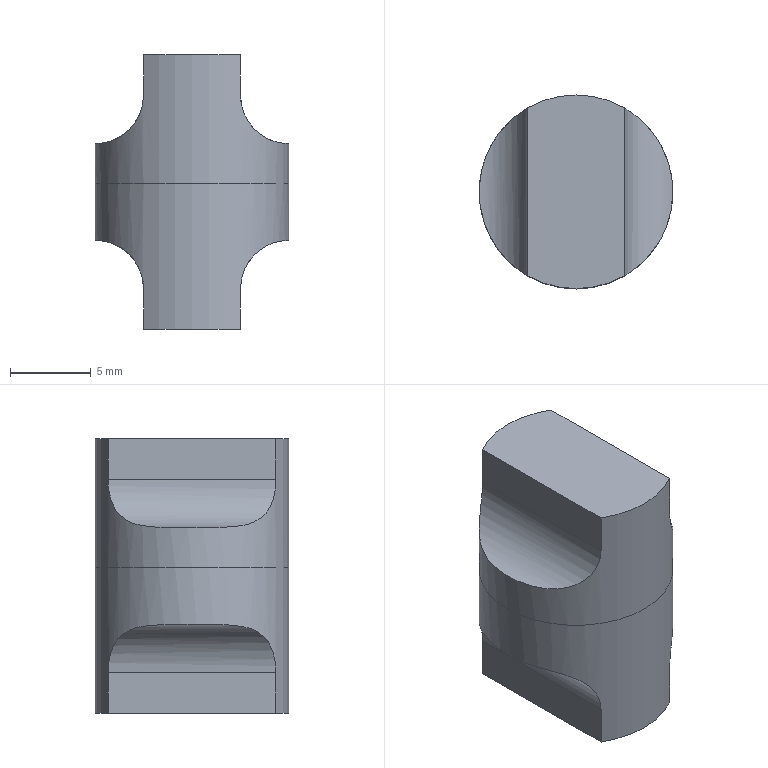NC program | NX | posted with a generic post | part box 12 x 12 x 17 mm
Lines 1 to 1209 of 2569:
N10 G17 G21 G94 G90
(PLANAR_MILL , TOOL : D8开粗)
N12 T01 M6
N14 G53
N16 G17 G0 G90 X0. Y-12.196 S2000 M3
N18 G43 Z20. H1
N20 Z2.05
N22 G94 G1 Z0.05 F800.
N24 Y-5.196
N26 Y5.196
N28 Y12.196
N30 Z2.05
N32 G0 Z20.
(ADAPTIVE_MILLING , TOOL : D8开粗)
N34 X-16.483 Y0.108 S3000
N36 Z-8.5
N38 G1 X-16.333 Z-9.437 F1000.
N40 X-16.183 Z-9.808
N42 X-16.033 Z-10.08
N44 X-15.883 Z-10.3
N46 X-15.733 Z-10.484
N48 X-15.583 Y0.107 Z-10.642
N50 X-15.433 Z-10.78
N52 X-15.283 Z-10.9
N54 X-15.133 Z-11.005
N56 X-14.983 Z-11.098
N58 X-14.833 Z-11.179
N60 X-14.683 Z-11.25
N62 X-14.533 Z-11.31
N64 X-14.383 Z-11.362
N66 X-14.233 Z-11.405
N68 X-14.083 Z-11.439
N70 X-13.933 Z-11.466
N72 X-13.783 Z-11.485
N74 X-13.633 Z-11.496
N76 X-13.483 Z-11.5
N78 X-12.219
N80 G3 X-11.455 Y0.65 R0.809
N82 G1 X-11.311 Y1.182
N84 X-11.182 Y1.718
N86 G2 X-10.176 Y4.671 R15.023
N88 X-4.959 Y10.014 R11.386
N90 X-11.055 Y-1.588 R-11.172
N92 X-10.974 Y1.151 R9.54
N94 X-8.589 Y6.675 R12.062
N96 X8.313 Y6.997 R10.886
N98 X-10.527 Y-2.655 R-10.862
N100 X-10.588 Y1.538 R10.069
N102 X-6.776 Y8.1 R11.189
N104 X8.091 Y6.77 R10.555
N106 X6.739 Y-8.116 R10.555
N108 X-9.934 Y-3.527 R10.537
N110 X-10.226 Y1.752 R9.997
N112 X-5.977 Y8.319 R10.75
N114 X7.767 Y-6.659 R10.238
N116 X-9.264 Y-4.321 R10.22
N118 X-10.105 Y-0.867 R9.526
N120 X-10.122 Y0.747 R16.055
N122 G1 X-9.903 Y2.224
N124 X-9.47 Y3.652
N126 X-8.832 Y5.001
N128 X-8.003 Y6.243
N130 X-7.001 Y7.349
N132 G2 X-5.014 Y8.825 R12.775
N134 X-2.455 Y9.848 R11.845
N136 X1.637 Y10.017 R10.974
N138 X5.463 Y8.555 R10.975
N140 G1 X6.252 Y7.996
N142 X7.381 Y6.967
N144 X8.343 Y5.78
N146 X9.116 Y4.463
N148 X9.682 Y3.045
N150 X10.03 Y1.558
N152 X10.15 Y0.036
N154 X10.04 Y-1.487
N156 X9.704 Y-2.976
N158 X9.147 Y-4.398
N160 X8.384 Y-5.721
N162 X7.431 Y-6.914
N164 G2 X5.936 Y-8.229 R14.803
N166 X4.246 Y-9.219 R14.74
N168 G1 X2.885 Y-9.731
N170 X1.467 Y-10.043
N172 X0.019 Y-10.15
N174 X-1.429 Y-10.049
N176 X-2.848 Y-9.742
N178 X-4.209 Y-9.236
N180 G2 X-5.849 Y-8.295 R16.559
N182 G1 X-7.003 Y-7.347
N184 X-8.005 Y-6.241
N186 X-8.833 Y-4.999
N188 X-9.471 Y-3.65
N190 X-9.904 Y-2.222
N192 X-10.123 Y-0.746
N194 X-10.122 Y0.029
N196 G3 X-10.746 Y0.816 R0.808
N198 G1 X-12.079 Y1.127
N200 X-12.225 Y1.162 Z-11.496
N202 X-12.371 Y1.196 Z-11.485
N204 X-12.517 Y1.23 Z-11.466
N206 X-12.663 Y1.264 Z-11.439
N208 X-12.809 Y1.298 Z-11.405
N210 X-12.955 Y1.333 Z-11.362
N212 X-13.101 Y1.367 Z-11.31
N214 X-13.247 Y1.401 Z-11.25
N216 X-13.393 Y1.435 Z-11.179
N218 X-13.539 Y1.469 Z-11.098
N220 X-13.686 Y1.504 Z-11.005
N222 X-13.832 Y1.538 Z-10.9
N224 X-13.978 Y1.572 Z-10.78
N226 X-14.124 Y1.606 Z-10.642
N228 X-14.27 Y1.64 Z-10.484
N230 X-14.416 Y1.674 Z-10.3
N232 X-14.562 Y1.709 Z-10.08
N234 X-14.708 Y1.743 Z-9.808
N236 X-14.854 Y1.777 Z-9.437
N238 X-15. Y1.811 Z-8.5
N240 G0 Z20.
N242 X-10.3 Y-11.092
N244 Z-1.792
N246 G1 X-10.195 Y-10.985 Z-2.728
N248 X-10.089 Y-10.879 Z-3.099
N250 X-9.983 Y-10.772 Z-3.372
N252 X-9.878 Y-10.666 Z-3.592
N254 X-9.772 Y-10.559 Z-3.776
N256 X-9.667 Y-10.453 Z-3.934
N258 X-9.561 Y-10.346 Z-4.071
N260 X-9.455 Y-10.24 Z-4.192
N262 X-9.35 Y-10.133 Z-4.297
N264 X-9.244 Y-10.027 Z-4.39
N266 X-9.139 Y-9.92 Z-4.471
N268 X-9.033 Y-9.814 Z-4.541
N270 X-8.927 Y-9.707 Z-4.602
N272 X-8.822 Y-9.601 Z-4.653
N274 X-8.716 Y-9.494 Z-4.696
N276 X-8.611 Y-9.388 Z-4.731
N278 X-8.505 Y-9.281 Z-4.758
N280 X-8.399 Y-9.175 Z-4.777
N282 X-8.294 Y-9.068 Z-4.788
N284 X-8.188 Y-8.962 Z-4.792
N286 X-7.328 Y-8.094
N288 G3 X-7.296 Y-6.991 R0.808
N290 G2 X-8.074 Y-5.822 R7.553
N292 X-9.766 Y0.923 R10.805
N294 X-7.99 Y5.701 R10.308
N296 X-7.292 Y6.995 R3.699
N298 G3 X-8.256 Y8.237 R0.8
N300 G1 X-8.458 Y8.097 Z-4.776
N302 X-8.645 Y7.939 Z-4.761
N304 X-9.494 Y7.236 Z-4.692
N306 X-10.032 Y6.789 F10000.
N308 G3 X-10.322 Y6.183 R0.803
N310 G1 X-10.474 Y-6.011
N312 G3 X-10.166 Y-6.651 R0.802
N314 G1 X-9.58 Y-7.109
N316 X-8.578 Y-7.884 Z-4.771 F1000.
N318 X-8.434 Y-7.959 Z-4.781
N320 X-8.279 Y-8.005 Z-4.792
N322 G3 X-7.444 Y-6.822 R0.8
N324 G2 X-9.296 Y-2.127 R16.929
N326 X-8.227 Y4.755 R10.197
N328 G1 X-8.158 Y4.969
N330 G3 X-8.686 Y5.848 R0.8
N332 X-9.443 Y5.725 Z-4.742 R0.833
N334 G1 X-10.115 Y5.3 Z-4.692
N336 X-10.815 Y4.858 F10000.
N338 G3 X-11.187 Y4.157 R0.801
N340 G1 X-10.895 Y-5.268
N342 G3 X-10.57 Y-5.888 R0.802
N344 G1 X-9.862 Y-6.408
N346 X-9.047 Y-7.002 Z-4.755 F1000.
N348 G3 X-8.487 Y-7.112 Z-4.792 R0.801
N350 X-7.866 Y-6.08 R0.8
N352 G2 X-8.911 Y-2.674 R47.106
N354 X-8.355 Y3.815 R10.582
N356 G3 X-8.214 Y4.419 R1.722
N358 G2 X-7.965 Y5.768 R4.245
N360 G3 X-9.236 Y6.63 R0.8
N362 G1 X-9.375 Y6.479 Z-4.779
N364 X-9.487 Y6.307 Z-4.766
N366 X-10.118 Y5.308 Z-4.692
N368 X-10.368 Y4.915 F10000.
N370 X-10.609 Y4.516
N372 X-10.66 Y4.361
N374 X-10.681 Y4.2
N376 X-10.842 Y-3.699
N378 G3 X-10.702 Y-4.168 R0.81
N380 G1 X-10.169 Y-4.945
N382 X-9.847 Y-5.421 Z-4.728 F1000.
N384 X-9.513 Y-5.889 Z-4.764
N386 G3 X-9.14 Y-6.119 Z-4.792 R0.834
N388 X-8.126 Y-5.267 R0.8
N390 X-8.641 Y-2.873 R41.453
N392 G2 X-8.32 Y3.115 R11.676
N394 G3 X-8.214 Y4.324 R3.422
N396 X-9.006 Y5.124 R0.8
N398 X-9.673 Y4.784 Z-4.743 R0.83
N400 G1 X-10.199 Y4.161 Z-4.692
N402 X-11.129 Y3.059 F10000.
N404 G3 X-11.318 Y2.532 R0.806
N406 G1 X-11.24 Y-3.376
N408 G3 X-11.065 Y-3.865 R0.808
N410 G1 X-10.165 Y-4.99
N412 X-9.514 Y-5.795 Z-4.757 F1000.
N414 G3 X-9.029 Y-6.044 Z-4.792 R0.802
N416 X-8.136 Y-5.168 R0.8
N418 X-8.547 Y-2.088 R101.131
N420 G2 X-8.216 Y2.562 R14.182
N422 G1 X-8.214 Y3.624
N424 G3 X-9.009 Y4.424 R0.8
N426 X-9.674 Y4.082 Z-4.743 R0.83
N428 G1 X-10.199 Y3.457 Z-4.692
N430 X-11.131 Y2.347 F10000.
N432 G3 X-11.318 Y1.832 R0.807
N434 G1 Y-2.626
N436 G3 X-11.131 Y-3.14 R0.807
N438 G1 X-10.215 Y-4.231
N440 X-9.579 Y-4.98 Z-4.753 F1000.
N442 G3 X-9.034 Y-5.218 Z-4.792 R0.8
N444 X-8.214 Y-4.418 R0.8
N446 X-8.366 Y-1.622 R52.778
N448 G2 X-8.214 Y1.139 R16.802
N450 G1 Y2.614
N452 G3 X-9.627 Y3.128 R0.8
N454 X-9.82 Y2.735 Z-4.764 R1.147
N456 G1 X-10.201 Y1.648 Z-4.692
N458 X-10.748 Y0.08 F10000.
N460 X-11.318 Y-2.176
N462 G3 X-11.12 Y-2.925 R0.801
N464 G1 X-10.216 Y-3.87
N466 X-9.881 Y-4.222 Z-4.722 F1000.
N468 X-9.54 Y-4.567 Z-4.753
N470 G3 X-8.969 Y-4.767 Z-4.792 R0.8
N472 X-8.214 Y-3.968 R0.8
N474 G1 Y1.157
N476 G3 X-9.145 Y1.955 R0.808
N478 G1 X-10.205 Y1.792
N480 X-10.353 Y1.769 Z-4.788
N482 X-10.502 Y1.746 Z-4.777
N484 X-10.65 Y1.723 Z-4.758
N486 X-10.798 Y1.701 Z-4.731
N488 X-10.946 Y1.678 Z-4.696
N490 X-11.095 Y1.655 Z-4.653
N492 X-11.243 Y1.632 Z-4.602
N494 X-11.391 Y1.609 Z-4.541
N496 X-11.539 Y1.586 Z-4.471
N498 X-11.688 Y1.563 Z-4.39
N500 X-11.836 Y1.541 Z-4.297
N502 X-11.984 Y1.518 Z-4.192
N504 X-12.132 Y1.495 Z-4.071
N506 X-12.281 Y1.472 Z-3.934
N508 X-12.429 Y1.449 Z-3.776
N510 X-12.577 Y1.426 Z-3.592
N512 X-12.725 Y1.404 Z-3.372
N514 X-12.874 Y1.381 Z-3.099
N516 X-13.022 Y1.358 Z-2.728
N518 X-13.17 Y1.335 Z-1.792
N520 G0 Z20.
N522 X-6.462 Y-13.661
N524 Z-0.833
N526 G1 X-6.394 Y-13.528 Z-1.77
N528 X-6.325 Y-13.394 Z-2.141
N530 X-6.256 Y-13.261 Z-2.414
N532 X-6.187 Y-13.128 Z-2.633
N534 X-6.118 Y-12.995 Z-2.818
N536 X-6.049 Y-12.861 Z-2.976
N538 X-5.98 Y-12.728 Z-3.113
N540 X-5.911 Y-12.595 Z-3.233
N542 X-5.842 Y-12.462 Z-3.339
N544 X-5.774 Y-12.328 Z-3.431
N546 X-5.705 Y-12.195 Z-3.512
N548 X-5.636 Y-12.062 Z-3.583
N550 X-5.567 Y-11.929 Z-3.644
N552 X-5.498 Y-11.795 Z-3.695
N554 X-5.429 Y-11.662 Z-3.738
N556 X-5.36 Y-11.529 Z-3.773
N558 X-5.291 Y-11.396 Z-3.799
N560 X-5.222 Y-11.262 Z-3.818
N562 X-5.153 Y-11.129 Z-3.83
N564 X-5.085 Y-10.996 Z-3.833
N566 X-4.55 Y-9.962
N568 G3 X-4.914 Y-8.864 R0.808
N570 G2 X-7.438 Y-5.866 R4.709
N572 X-7.973 Y-1.991 R13.945
N574 X-7.993 Y3.683 R135.06
N576 X-7.375 Y5.808 R6.277
N578 X-5.432 Y8.574 R4.233
N580 G1 X-4.992 Y8.836
N582 G3 X-4.864 Y10.203 R0.8
N584 X-5.461 Y10.351 Z-3.794 R0.845
N586 G1 X-6.421 Y10.291 Z-3.733
N588 X-7.789 Y10.204 F10000.
N590 G3 X-8.454 Y9.763 R0.801
N592 G1 X-8.901 Y8.875
N594 X-9.334 Y7.98
N596 G3 X-10.118 Y5.441 R11.255
N598 X-10.403 Y2.107 R15.175
N600 G1 X-10.184 Y-6.447
N602 G3 X-9.835 Y-7.087 R0.802
N604 G1 X-8.771 Y-7.813
N606 X-7.816 Y-8.459 Z-3.806 F1000.
N608 G3 X-7.396 Y-8.567 Z-3.833 R0.807
N610 X-6.722 Y-7.374 R0.8
N612 G2 X-7.482 Y-5.23 R4.771
N614 X-7.807 Y1.332 R51.098
N616 X-7.464 Y4.651 R11.067
N618 X-7.374 Y5.812 R3.596
N620 G3 X-8.517 Y6.738 R0.8
N622 X-8.903 Y6.328 Z-3.798 R1.014
N624 G1 X-9.452 Y5.467 Z-3.733
N626 X-9.741 Y5.02 F10000.
N628 X-10.018 Y4.566
N630 X-10.07 Y4.408
N632 X-10.09 Y4.244
N634 X-10.195 Y-3.687
N636 G3 X-10.037 Y-4.174 R0.809
N638 G1 X-9.465 Y-4.945
N640 X-8.875 Y-5.731 Z-3.795 F1000.
N642 G3 X-8.346 Y-6.001 Z-3.833 R0.8
N644 X-7.479 Y-5.255 R0.8
N646 X-7.565 Y-1.288 R67.895
N648 G2 X-7.534 Y2.609 R34.546
N650 G3 X-7.463 Y4.681 R12.448
N652 X-8.839 Y5.235 R0.8
N654 X-9.068 Y4.809 Z-3.803 R1.097
N656 G1 X-9.45 Y3.772 Z-3.733
N658 X-9.718 Y3.055 F10000.
N660 X-9.975 Y2.333
N662 X-9.997 Y2.146
N664 Y-1.924
N666 X-9.983 Y-2.064
N668 X-9.948 Y-2.201
N670 X-9.46 Y-3.523
N672 X-9.222 Y-4.177 Z-3.777 F1000.
N674 X-8.973 Y-4.827 Z-3.821
N676 X-8.859 Y-4.991 Z-3.833
N678 G3 X-7.463 Y-4.458 R0.8
N680 G1 Y3.217
N682 G3 X-8.254 Y4.025 R0.808
N684 G1 X-9.454 Y4.05
N686 X-9.604 Y4.053 Z-3.83
N688 X-9.754 Y4.056 Z-3.818
N690 X-9.904 Y4.059 Z-3.799
N692 X-10.054 Y4.063 Z-3.773
N694 X-10.204 Y4.066 Z-3.738
N696 X-10.354 Y4.069 Z-3.695
N698 X-10.504 Y4.072 Z-3.644
N700 X-10.654 Y4.075 Z-3.583
N702 X-10.804 Y4.078 Z-3.512
N704 X-10.954 Y4.081 Z-3.431
N706 X-11.104 Y4.085 Z-3.339
N708 X-11.254 Y4.088 Z-3.233
N710 X-11.404 Y4.091 Z-3.113
N712 X-11.553 Y4.094 Z-2.976
N714 X-11.703 Y4.097 Z-2.818
N716 X-11.853 Y4.1 Z-2.633
N718 X-12.003 Y4.103 Z-2.414
N720 X-12.153 Y4.107 Z-2.141
N722 X-12.303 Y4.11 Z-1.77
N724 X-12.453 Y4.113 Z-0.833
N726 G0 Z20.
N728 X-5.602 Y-14.052
N730 Z0.125
N732 G1 X-5.547 Y-13.912 Z-0.812
N734 X-5.493 Y-13.773 Z-1.183
N736 X-5.438 Y-13.633 Z-1.455
N738 X-5.383 Y-13.494 Z-1.675
N740 X-5.328 Y-13.354 Z-1.859
N742 X-5.273 Y-13.214 Z-2.017
N744 X-5.218 Y-13.075 Z-2.155
N746 X-5.164 Y-12.935 Z-2.275
N748 X-5.109 Y-12.795 Z-2.38
N750 X-5.054 Y-12.656 Z-2.473
N752 X-4.999 Y-12.516 Z-2.554
N754 X-4.944 Y-12.377 Z-2.625
N756 X-4.89 Y-12.237 Z-2.685
N758 X-4.835 Y-12.097 Z-2.737
N760 X-4.78 Y-11.958 Z-2.78
N762 X-4.725 Y-11.818 Z-2.814
N764 X-4.67 Y-11.679 Z-2.841
N766 X-4.615 Y-11.539 Z-2.86
N768 X-4.561 Y-11.399 Z-2.871
N770 X-4.506 Y-11.26 Z-2.875
N772 X-4.06 Y-10.124
N774 G3 X-4.444 Y-9.11 R0.808
N776 G2 X-6.383 Y-7.639 R4.863
N778 X-7.201 Y-5.205 R4.521
N780 X-7.245 Y4.22 R327.967
N782 G3 X-7.198 Y5.255 R3.972
N784 G2 X-6.34 Y7.696 R4.488
N786 X-4.434 Y9.12 R4.988
N788 G3 X-4.575 Y10.602 R0.8
N790 X-5.062 Y10.604 Z-2.844 R1.089
N792 G1 X-6.152 Y10.453 Z-2.775
N794 X-7.44 Y10.274 F10000.
N796 G3 X-7.896 Y10.047 R0.809
N798 G1 X-8.381 Y9.551
N800 G3 X-8.779 Y8.879 R2.386
N802 X-9.296 Y7.276 R10.148
N804 X-9.478 Y6.003 R11.42
N806 X-9.66 Y3.03 R31.031
N808 G1 X-9.732 Y-2.721
N810 X-9.717 Y-2.876
N812 X-9.676 Y-3.026
N814 X-9.183 Y-4.265
N816 X-8.702 Y-5.464 Z-2.856 F1000.
N818 X-8.624 Y-5.592 Z-2.866
N820 X-8.525 Y-5.705 Z-2.875
N822 G3 X-7.198 Y-5.255 R0.8
N824 G1 X-7.174 Y-5.029
N826 Y4.821
N828 G3 X-7.758 Y5.597 R0.808
N830 G1 X-9.11 Y5.987
N832 X-9.254 Y6.029 Z-2.871
N834 X-9.398 Y6.07 Z-2.86
N836 X-9.542 Y6.112 Z-2.841
N838 X-9.686 Y6.154 Z-2.814
N840 X-9.83 Y6.195 Z-2.78
N842 X-9.974 Y6.237 Z-2.737
N844 X-10.119 Y6.278 Z-2.685
N846 X-10.263 Y6.32 Z-2.625
N848 X-10.407 Y6.361 Z-2.554
N850 X-10.551 Y6.403 Z-2.473
N852 X-10.695 Y6.445 Z-2.38
N854 X-10.839 Y6.486 Z-2.275
N856 X-10.983 Y6.528 Z-2.155
N858 X-11.127 Y6.569 Z-2.017
N860 X-11.272 Y6.611 Z-1.859
N862 X-11.416 Y6.652 Z-1.675
N864 X-11.56 Y6.694 Z-1.455
N866 X-11.704 Y6.736 Z-1.183
N868 X-11.848 Y6.777 Z-0.812
N870 X-11.992 Y6.819 Z0.125
N872 G0 Z20.
N874 X10.317 Y11.075
N876 Z-1.792
N878 G1 X10.211 Y10.969 Z-2.728
N880 X10.105 Y10.863 Z-3.099
N882 X9.999 Y10.757 Z-3.372
N884 X9.892 Y10.651 Z-3.592
N886 X9.786 Y10.545 Z-3.776
N888 X9.68 Y10.439 Z-3.934
N890 X9.574 Y10.334 Z-4.071
N892 X9.468 Y10.228 Z-4.192
N894 X9.361 Y10.122 Z-4.297
N896 X9.255 Y10.016 Z-4.39
N898 X9.149 Y9.91 Z-4.471
N900 X9.043 Y9.804 Z-4.541
N902 X8.936 Y9.698 Z-4.602
N904 X8.83 Y9.592 Z-4.653
N906 X8.724 Y9.486 Z-4.696
N908 X8.618 Y9.38 Z-4.731
N910 X8.512 Y9.274 Z-4.758
N912 X8.405 Y9.169 Z-4.777
N914 X8.299 Y9.063 Z-4.788
N916 X8.193 Y8.957 Z-4.792
N918 X7.331 Y8.097
N920 G3 X7.296 Y6.991 R0.808
N922 G2 X8.159 Y5.677 R8.398
N924 X9.615 Y-1.949 R10.578
N926 X7.996 Y-5.688 R10.119
N928 G1 X7.976 Y-5.734
N930 G3 X8.535 Y-6.752 R0.8
N932 X9.255 Y-6.593 Z-4.744 R0.838
N934 G1 X9.936 Y-6.121 Z-4.692
N936 X10.662 Y-5.619 F10000.
N938 G3 X11.005 Y-4.923 R0.801
N940 G1 X10.474 Y6.011
N942 G3 X10.179 Y6.593 R0.803
N944 G1 X9.608 Y7.056
N946 X8.596 Y7.872 Z-4.773 F1000.
N948 X8.469 Y7.944 Z-4.782
N950 X8.332 Y7.994 Z-4.792
N952 G3 X7.444 Y6.822 R0.8
N954 G2 X9.279 Y2.209 R17.045
N956 X8.304 Y-4.594 R9.947
N958 G1 X8.157 Y-4.976
N960 G3 X8.684 Y-5.845 R0.8
N962 X9.441 Y-5.726 Z-4.742 R0.833
N964 G1 X10.115 Y-5.303 Z-4.692
N966 X10.515 Y-5.056 F10000.
N968 X10.907 Y-4.797
N970 G3 X11.186 Y-4.165 R0.802
N972 G1 X10.895 Y5.268
N974 G3 X10.57 Y5.888 R0.802
N976 G1 X9.862 Y6.409
N978 X9.047 Y7.002 Z-4.755 F1000.
N980 G3 X8.487 Y7.111 Z-4.792 R0.801
N982 X7.866 Y6.08 R0.8
N984 G2 X8.898 Y2.733 R49.952
N986 X8.351 Y-3.828 R10.609
N988 G3 X8.214 Y-4.419 R1.641
N990 G2 X7.441 Y-6.826 R4.467
N992 G1 X7.292 Y-6.995
N994 G3 X8.295 Y-8.216 R0.8
N996 G1 X8.562 Y-8.01 Z-4.77
N998 X8.817 Y-7.789 Z-4.749
N1000 X9.517 Y-7.195 Z-4.692
N1002 X9.83 Y-6.934 F10000.
N1004 X10.132 Y-6.659
N1006 G3 X10.322 Y-6.183 R0.809
N1008 G1 X10.842 Y3.699
N1010 G3 X10.699 Y4.199 R0.808
N1012 G1 X10.169 Y4.96
N1014 X9.844 Y5.431 Z-4.728 F1000.
N1016 X9.508 Y5.894 Z-4.764
N1018 G3 X9.129 Y6.122 Z-4.792 R0.834
N1020 X8.126 Y5.267 R0.8
N1022 X8.649 Y2.833 R43.85
N1024 G2 X8.322 Y-3.107 R11.641
N1026 G3 X8.214 Y-4.347 R3.499
N1028 X9.006 Y-5.147 R0.8
N1030 X9.673 Y-4.806 Z-4.743 R0.83
N1032 G1 X10.199 Y-4.184 Z-4.692
N1034 X11.129 Y-3.081 F10000.
N1036 G3 X11.318 Y-2.555 R0.806
N1038 G1 X11.24 Y3.376
N1040 G3 X11.065 Y3.865 R0.808
N1042 G1 X10.165 Y4.99
N1044 X9.514 Y5.795 Z-4.757 F1000.
N1046 G3 X9.029 Y6.044 Z-4.792 R0.802
N1048 X8.136 Y5.168 R0.8
N1050 X8.551 Y2.048 R110.796
N1052 G2 X8.216 Y-2.567 R14.229
N1054 G1 X8.214 Y-3.598
N1056 G3 X9.009 Y-4.398 R0.8
N1058 X9.674 Y-4.056 Z-4.743 R0.83
N1060 G1 X10.199 Y-3.431 Z-4.692
N1062 X11.131 Y-2.321 F10000.
N1064 G3 X11.318 Y-1.806 R0.807
N1066 G1 Y2.625
N1068 G3 X11.131 Y3.14 R0.807
N1070 G1 X10.215 Y4.23
N1072 X9.579 Y4.98 Z-4.753 F1000.
N1074 G3 X9.034 Y5.217 Z-4.792 R0.8
N1076 X8.214 Y4.417 R0.8
N1078 X8.366 Y1.606 R55.27
N1080 G2 X8.214 Y-1.136 R16.703
N1082 G1 Y-2.611
N1084 G3 X9.627 Y-3.125 R0.8
N1086 X9.82 Y-2.732 Z-4.764 R1.147
N1088 G1 X10.201 Y-1.645 Z-4.692
N1090 X10.748 Y-0.077 F10000.
N1092 X11.318 Y2.2
N1094 G3 X11.12 Y2.947 R0.801
N1096 G1 X10.216 Y3.893
N1098 X9.882 Y4.245 Z-4.722 F1000.
N1100 X9.54 Y4.591 Z-4.753
N1102 G3 X8.97 Y4.791 Z-4.792 R0.8
N1104 X8.214 Y3.992 R0.8
N1106 G1 Y-1.158
N1108 G3 X9.145 Y-1.956 R0.808
N1110 G1 X10.205 Y-1.793
N1112 X10.353 Y-1.77 Z-4.788
N1114 X10.502 Y-1.747 Z-4.777
N1116 X10.65 Y-1.724 Z-4.758
N1118 X10.798 Y-1.702 Z-4.731
N1120 X10.946 Y-1.679 Z-4.696
N1122 X11.095 Y-1.656 Z-4.653
N1124 X11.243 Y-1.633 Z-4.602
N1126 X11.391 Y-1.61 Z-4.541
N1128 X11.539 Y-1.587 Z-4.471
N1130 X11.688 Y-1.564 Z-4.39
N1132 X11.836 Y-1.542 Z-4.297
N1134 X11.984 Y-1.519 Z-4.192
N1136 X12.132 Y-1.496 Z-4.071
N1138 X12.281 Y-1.473 Z-3.934
N1140 X12.429 Y-1.45 Z-3.776
N1142 X12.577 Y-1.427 Z-3.592
N1144 X12.725 Y-1.405 Z-3.372
N1146 X12.874 Y-1.382 Z-3.099
N1148 X13.022 Y-1.359 Z-2.728
N1150 X13.17 Y-1.336 Z-1.792
N1152 G0 Z20.
N1154 X6.474 Y13.676
N1156 Z-0.833
N1158 G1 X6.407 Y13.542 Z-1.77
N1160 X6.339 Y13.409 Z-2.141
N1162 X6.272 Y13.275 Z-2.414
N1164 X6.204 Y13.141 Z-2.633
N1166 X6.137 Y13.007 Z-2.818
N1168 X6.069 Y12.873 Z-2.976
N1170 X6.002 Y12.739 Z-3.113
N1172 X5.934 Y12.605 Z-3.233
N1174 X5.867 Y12.471 Z-3.339
N1176 X5.799 Y12.337 Z-3.431
N1178 X5.732 Y12.203 Z-3.512
N1180 X5.664 Y12.069 Z-3.583
N1182 X5.597 Y11.935 Z-3.644
N1184 X5.529 Y11.801 Z-3.695
N1186 X5.462 Y11.667 Z-3.738
N1188 X5.394 Y11.533 Z-3.773
N1190 X5.327 Y11.399 Z-3.799
N1192 X5.259 Y11.265 Z-3.818
N1194 X5.192 Y11.131 Z-3.83
N1196 X5.124 Y10.998 Z-3.833
N1198 X4.591 Y9.939
N1200 G3 X4.947 Y8.855 R0.808
N1202 G2 X7.453 Y5.807 R4.754
N1204 X7.968 Y1.903 R14.463
N1206 X7.992 Y-3.671 R140.433
N1208 X7.377 Y-5.8 R6.241
N1210 X5.375 Y-8.607 R4.238
N1212 G1 X4.914 Y-8.864
N1214 G3 X4.821 Y-10.25 R0.8
N1216 X5.39 Y-10.378 Z-3.796 R0.858
N1218 G1 X6.385 Y-10.315 Z-3.733
N1220 X7.71 Y-10.233 F10000.
N1222 G3 X8.376 Y-9.792 R0.801
N1224 G1 X9.035 Y-8.453
N1226 G3 X9.569 Y-7.063 R13.559
N1228 G1 X10.013 Y-5.639
N1230 G3 X10.477 Y-2.228 R12.817
N1232 X10.39 Y1.749 R95.02
N1234 G1 X10.183 Y6.446
N1236 G3 X9.838 Y7.069 R0.802
N1238 G1 X8.775 Y7.802
N1240 X7.818 Y8.457 Z-3.806 F1000.
N1242 G3 X7.405 Y8.567 Z-3.833 R0.808
N1244 X6.721 Y7.374 R0.8
N1246 G2 X7.482 Y5.23 R4.769
N1248 X7.805 Y-1.662 R55.963
N1250 X7.463 Y-4.661 R11.247
N1252 X7.375 Y-5.809 R3.49
N1254 G3 X8.517 Y-6.735 R0.8
N1256 X8.903 Y-6.325 Z-3.798 R1.014
N1258 G1 X9.453 Y-5.464 Z-3.733
N1260 X9.742 Y-5.017 F10000.
N1262 X10.018 Y-4.563
N1264 X10.07 Y-4.405
N1266 X10.091 Y-4.241
N1268 X10.195 Y3.687
N1270 G3 X10.037 Y4.174 R0.809
N1272 G1 X9.465 Y4.945
N1274 X8.875 Y5.731 Z-3.795 F1000.
N1276 G3 X8.346 Y6.001 Z-3.833 R0.8
N1278 X7.479 Y5.255 R0.8
N1280 X7.564 Y1.109 R74.343
N1282 G2 X7.522 Y-2.688 R31.7
N1284 G3 X7.463 Y-4.665 R12.516
N1286 X8.839 Y-5.219 R0.8
N1288 X9.068 Y-4.793 Z-3.803 R1.097
N1290 G1 X9.45 Y-3.756 Z-3.733
N1292 X9.718 Y-3.038 F10000.
N1294 X9.975 Y-2.317
N1296 X9.997 Y-2.13
N1298 Y1.849
N1300 X9.983 Y1.989
N1302 X9.948 Y2.126
N1304 X9.46 Y3.448
N1306 X9.222 Y4.102 Z-3.777 F1000.
N1308 X8.973 Y4.752 Z-3.821
N1310 X8.859 Y4.916 Z-3.833
N1312 G3 X7.463 Y4.383 R0.8
N1314 G1 Y-3.192
N1316 G3 X8.256 Y-4. R0.808
N1318 G1 X9.454 Y-4.021
N1320 X9.604 Y-4.024 Z-3.83
N1322 X9.754 Y-4.026 Z-3.818
N1324 X9.904 Y-4.029 Z-3.799
N1326 X10.054 Y-4.032 Z-3.773
N1328 X10.204 Y-4.034 Z-3.738
N1330 X10.354 Y-4.037 Z-3.695
N1332 X10.504 Y-4.04 Z-3.644
N1334 X10.654 Y-4.042 Z-3.583
N1336 X10.804 Y-4.045 Z-3.512
N1338 X10.954 Y-4.048 Z-3.431
N1340 X11.104 Y-4.05 Z-3.339
N1342 X11.254 Y-4.053 Z-3.233
N1344 X11.404 Y-4.056 Z-3.113
N1346 X11.554 Y-4.058 Z-2.976
N1348 X11.704 Y-4.061 Z-2.818
N1350 X11.854 Y-4.063 Z-2.633
N1352 X12.004 Y-4.066 Z-2.414
N1354 X12.154 Y-4.069 Z-2.141
N1356 X12.304 Y-4.071 Z-1.77
N1358 X12.453 Y-4.074 Z-0.833
N1360 G0 Z20.
N1362 X5.429 Y14.13
N1364 Z0.125
N1366 G1 X5.376 Y13.989 Z-0.812
N1368 X5.324 Y13.849 Z-1.183
N1370 X5.272 Y13.708 Z-1.455
N1372 X5.219 Y13.567 Z-1.675
N1374 X5.167 Y13.427 Z-1.859
N1376 X5.114 Y13.286 Z-2.017
N1378 X5.062 Y13.146 Z-2.155
N1380 X5.01 Y13.005 Z-2.275
N1382 X4.957 Y12.865 Z-2.38
N1384 X4.905 Y12.724 Z-2.473
N1386 X4.852 Y12.584 Z-2.554
N1388 X4.8 Y12.443 Z-2.625
N1390 X4.748 Y12.302 Z-2.685
N1392 X4.695 Y12.162 Z-2.737
N1394 X4.643 Y12.021 Z-2.78
N1396 X4.59 Y11.881 Z-2.814
N1398 X4.538 Y11.74 Z-2.841
N1400 X4.486 Y11.6 Z-2.86
N1402 X4.433 Y11.459 Z-2.871
N1404 X4.381 Y11.319 Z-2.875
N1406 X3.946 Y10.152
N1408 G3 X4.35 Y9.142 R0.808
N1410 G2 X6.365 Y7.66 R4.856
N1412 X7.201 Y5.205 R4.539
N1414 X7.244 Y-4.228 R328.464
N1416 G3 X7.198 Y-5.255 R3.958
N1418 G2 X6.382 Y-7.638 R4.479
N1420 X5.116 Y-8.766 R4.819
N1422 G1 X4.353 Y-9.141
N1424 G3 X4.549 Y-10.643 R0.8
N1426 X4.971 Y-10.63 Z-2.848 R1.171
N1428 G1 X6.128 Y-10.468 Z-2.775
N1430 X7.361 Y-10.295 F10000.
N1432 G3 X7.815 Y-10.069 R0.809
N1434 G1 X8.3 Y-9.572
N1436 G3 X8.7 Y-8.901 R2.41
N1438 G1 X9.008 Y-8.111
N1440 X9.304 Y-7.317
N1442 G3 X9.781 Y-4.328 R9.22
N1444 G1 X9.732 Y2.721
N1446 X9.716 Y2.867
N1448 X9.676 Y3.009
N1450 X9.184 Y4.256
N1452 X8.704 Y5.461 Z-2.856 F1000.
N1454 X8.628 Y5.587 Z-2.866
N1456 X8.532 Y5.699 Z-2.875
N1458 G3 X7.198 Y5.255 R0.8
N1460 G1 X7.174 Y5.029
N1462 Y-4.846
N1464 G3 X7.753 Y-5.621 R0.808
N1466 G1 X9.107 Y-6.021
N1468 X9.251 Y-6.063 Z-2.871
N1470 X9.395 Y-6.106 Z-2.86
N1472 X9.539 Y-6.148 Z-2.841
N1474 X9.683 Y-6.191 Z-2.814
N1476 X9.826 Y-6.233 Z-2.78
N1478 X9.97 Y-6.276 Z-2.737
N1480 X10.114 Y-6.318 Z-2.685
N1482 X10.258 Y-6.361 Z-2.625
N1484 X10.402 Y-6.403 Z-2.554
N1486 X10.546 Y-6.446 Z-2.473
N1488 X10.69 Y-6.488 Z-2.38
N1490 X10.833 Y-6.531 Z-2.275
N1492 X10.977 Y-6.573 Z-2.155
N1494 X11.121 Y-6.616 Z-2.017
N1496 X11.265 Y-6.658 Z-1.859
N1498 X11.409 Y-6.701 Z-1.675
N1500 X11.553 Y-6.743 Z-1.455
N1502 X11.697 Y-6.786 Z-1.183
N1504 X11.84 Y-6.828 Z-0.812
N1506 X11.984 Y-6.871 Z0.125
N1508 G0 Z20.
N1510 M5
(PLANAR_MILL_3 , TOOL : D6倒角刀)
N1512 T05 M6
N1514 G53
N1516 G17 G0 G90 X-4.7 Y-9.196 S3000 M3
N1518 G43 Z20. H5
N1520 Z0.
N1522 G94 G1 Z-2. F800.
N1524 Y-5.196
N1526 Y5.196
N1528 Y9.196
N1530 Z0.
N1532 G0 Z20.
N1534 X4.7
N1536 Z0.
N1538 G1 Z-2.
N1540 Y5.196
N1542 Y-5.196
N1544 Y-9.196
N1546 Z0.
N1548 G0 Z20.
(PLANAR_MILL_3_COPY , TOOL : D6倒角刀)
N1550 X7.464 Y-4.928
N1552 Z0.
N1554 G1 Z-2.
N1556 X4. Y-6.928
N1558 G2 X-4. Y-6.928 R8.
N1560 G1 X-7.464 Y-4.928
N1562 Z0.
N1564 G0 Z20.
N1566 Y4.928
N1568 Z0.
N1570 G1 Z-2.
N1572 X-4. Y6.928
N1574 G2 X4. Y6.928 R8.
N1576 G1 X7.464 Y4.928
N1578 Z0.
N1580 G0 Z20.
N1582 M5
(PLANAR_MILL_2 , TOOL : D8R3)
N1584 T07 M6
N1586 G53
N1588 G17 G0 G90 X-7. Y-11.196 S3000 M3
N1590 G43 Z20. H7
N1592 Z-3.5
N1594 G94 G1 Z-5.5 F600.
N1596 Y-5.196
N1598 Y5.196
N1600 Y11.196
N1602 Z-3.5
N1604 G0 Z3.
N1606 Y-11.196
N1608 Z-3.5
N1610 G1 Z-5.5
N1612 Y-5.196
N1614 Y5.196
N1616 Y11.196
N1618 Z-3.5
N1620 G0 Z3.
N1622 X7.
N1624 Z-3.5
N1626 G1 Z-5.5
N1628 Y5.196
N1630 Y-5.196
N1632 Y-11.196
N1634 Z-3.5
N1636 G0 Z3.
N1638 Y11.196
N1640 Z-3.5
N1642 G1 Z-5.5
N1644 Y5.196
N1646 Y-5.196
N1648 Y-11.196
N1650 Z-3.5
N1652 G0 Z20.
N1654 M5
(PLANAR_MILL_COPY , TOOL : D8精光)
N1656 T02 M6
N1658 G53
N1660 G17 G0 G90 X0. Y-12.196 S3000 M3
N1662 G43 Z20. H2
N1664 Z2.
N1666 G94 G1 Z0. F600.
N1668 Y-5.196
N1670 Y5.196
N1672 Y12.196
N1674 Z2.
N1676 G0 Z20.
(PLANAR_MILL_1 , TOOL : D8精光)
N1678 X-12. Y-2.
N1680 Z-9.5
N1682 G1 Z-11.5
N1684 G3 X-10. Y0. R2.
N1686 G2 X0. Y10. R10.
N1688 X-10. Y0. R-10.
N1690 G3 X-12. Y2. R2.
N1692 G1 Y-2.
N1694 G3 X-10. Y0. R2.
N1696 G2 X0. Y10. R10.
N1698 X-10. Y0. R-10.
N1700 G3 X-12. Y2. R2.
N1702 G1 Z-9.5
N1704 G0 Z20.
N1706 M5
(ADAPTIVE_MILLING_1 , TOOL : D8开粗)
N1708 T01 M6
N1710 G54
N1712 G17 G0 G90 X-16.448 Y-0.417 S2500 M3
N1714 G43 Z20. H1
N1716 Z0.6
N1718 G94 G1 X-16.3 Y-0.445 Z-0.337 F1000.
N1720 X-16.153 Y-0.472 Z-0.708
N1722 X-16.005 Y-0.5 Z-0.98
N1724 X-15.858 Y-0.527 Z-1.2
N1726 X-15.71 Y-0.555 Z-1.384
N1728 X-15.563 Y-0.582 Z-1.542
N1730 X-15.415 Y-0.61 Z-1.68
N1732 X-15.268 Y-0.637 Z-1.8
N1734 X-15.12 Y-0.665 Z-1.905
N1736 X-14.973 Y-0.692 Z-1.998
N1738 X-14.826 Y-0.72 Z-2.079
N1740 X-14.678 Y-0.747 Z-2.15
N1742 X-14.531 Y-0.775 Z-2.21
N1744 X-14.383 Y-0.802 Z-2.262
N1746 X-14.236 Y-0.83 Z-2.305
N1748 X-14.088 Y-0.857 Z-2.339
N1750 X-13.941 Y-0.885 Z-2.366
N1752 X-13.793 Y-0.912 Z-2.385
N1754 X-13.646 Y-0.94 Z-2.396
N1756 X-13.498 Y-0.967 Z-2.4
N1758 X-12.425 Y-1.168
N1760 G3 X-11.47 Y-0.424 R0.808
N1762 G2 X-10.815 Y2.952 R27.228
N1764 X4.713 Y10.132 R11.245
N1766 X-10.961 Y-2.078 R-11.169
N1768 X-7.035 Y8.283 R11.697
N1770 X-10.343 Y-3.282 R-10.862
N1772 X-4.224 Y9.671 R11.014
N1774 X-9.772 Y-3.935 R-10.549
N1776 X-2.316 Y9.969 R10.578
N1778 X-9.164 Y-4.511 R-10.23
N1780 X-0.706 Y9.885 R10.189
N1782 X-8.537 Y-4.988 R-9.905
N1784 X0.53 Y9.564 R9.821
N1786 X-7.879 Y-5.404 R-9.572
N1788 X1.485 Y9.119 R9.458
N1790 X-7.277 Y-5.649 R-9.231
N1792 X2.016 Y8.659 R9.096
N1794 X-6.548 Y-5.973 R-8.88
N1796 X2.531 Y8.147 R8.727
N1798 X-5.944 Y-6.076 R-8.519
N1800 X2.695 Y7.701 R8.351
N1802 X-5.209 Y-6.234 R-8.144
N1804 X-7.395 Y-3.242 R7.935
N1806 X-7.777 Y-2.16 R3.878
N1808 X-8.009 Y-1.015 R3.722
N1810 G1 X-8.098 Y-0.172
N1812 X-8.013 Y1.182
N1814 X-7.704 Y2.503
N1816 X-7.178 Y3.753
N1818 X-6.451 Y4.898
N1820 X-5.544 Y5.905
N1822 X-4.481 Y6.748
N1824 X-3.292 Y7.401
N1826 X-2.012 Y7.846
N1828 X-0.674 Y8.072
N1830 X0.654 Y8.073
N1832 X1.965 Y7.858
N1834 X3.223 Y7.431
N1836 X4.381 Y6.813
N1838 X5.424 Y6.015
N1840 X6.325 Y5.06
N1842 X7.06 Y3.971
N1844 X7.608 Y2.778
N1846 X7.957 Y1.513
N1848 X8.097 Y0.207
N1850 X8.024 Y-1.104
N1852 X7.74 Y-2.386
N1854 X7.253 Y-3.606
N1856 X6.575 Y-4.73
N1858 X5.702 Y-5.753
N1860 X4.672 Y-6.617
N1862 X3.513 Y-7.298
N1864 X2.258 Y-7.779
N1866 X0.94 Y-8.045
N1868 X-0.403 Y-8.09
N1870 X-1.736 Y-7.912
N1872 X-3.021 Y-7.516
N1874 X-4.222 Y-6.912
N1876 X-5.307 Y-6.119
N1878 X-6.246 Y-5.157
N1880 X-7.013 Y-4.053
N1882 X-7.591 Y-2.826
N1884 X-7.956 Y-1.52
N1886 X-8.011 Y-0.998
N1888 G3 X-8.726 Y-0.279 R0.808
N1890 G1 X-10.088 Y-0.129
N1892 X-10.237 Y-0.112 Z-2.396
N1894 X-10.386 Y-0.096 Z-2.385
N1896 X-10.535 Y-0.079 Z-2.366
N1898 X-10.684 Y-0.063 Z-2.339
N1900 X-10.833 Y-0.047 Z-2.305
N1902 X-10.983 Y-0.03 Z-2.262
N1904 X-11.132 Y-0.014 Z-2.21
N1906 X-11.281 Y0.003 Z-2.15
N1908 X-11.43 Y0.019 Z-2.079
N1910 X-11.579 Y0.036 Z-1.998
N1912 X-11.728 Y0.052 Z-1.905
N1914 X-11.877 Y0.069 Z-1.8
N1916 X-12.026 Y0.085 Z-1.68
N1918 X-12.175 Y0.102 Z-1.542
N1920 X-12.324 Y0.118 Z-1.384
N1922 X-12.473 Y0.134 Z-1.2
N1924 X-12.623 Y0.151 Z-0.98
N1926 X-12.772 Y0.167 Z-0.708
N1928 X-12.921 Y0.184 Z-0.337
N1930 X-13.07 Y0.2 Z0.6
N1932 G0 Z20.
N1934 X-13.125 Y-0.456
N1936 Z3.1
N1938 G1 X-12.975 Y-0.461 Z2.163
N1940 X-12.825 Y-0.466 Z1.792
N1942 X-12.676 Y-0.471 Z1.52
N1944 X-12.526 Y-0.477 Z1.3
N1946 X-12.376 Y-0.482 Z1.116
N1948 X-12.226 Y-0.487 Z0.958
N1950 X-12.076 Y-0.492 Z0.82
N1952 X-11.926 Y-0.498 Z0.7
N1954 X-11.776 Y-0.503 Z0.595
N1956 X-11.626 Y-0.508 Z0.502
N1958 X-11.476 Y-0.513 Z0.421
N1960 X-11.326 Y-0.519 Z0.35
N1962 X-11.176 Y-0.524 Z0.29
N1964 X-11.027 Y-0.529 Z0.238
N1966 X-10.877 Y-0.534 Z0.195
N1968 X-10.727 Y-0.54 Z0.161
N1970 X-10.577 Y-0.545 Z0.134
N1972 X-10.427 Y-0.55 Z0.115
N1974 X-10.277 Y-0.556 Z0.104
N1976 X-10.127 Y-0.561 Z0.1
N1978 X-8.868 Y-0.605
N1980 G3 X-8.059 Y-0.007 R0.808
N1982 G2 X-7.023 Y3.257 R13.424
N1984 X3.163 Y6.985 R7.792
N1986 X-7.295 Y-2.308 R-7.662
N1988 X-1.21 Y7.163 R7.685
N1990 X-6.166 Y-3.79 R-7.25
N1992 X0.698 Y6.784 R7.108
N1994 X-4.971 Y-4.622 R-6.804
N1996 X1.5 Y6.158 R6.595
N1998 X-3.455 Y-5.265 R-6.318
N2000 X1.187 Y5.682 R6.062
N2002 X5.641 Y-1.16 R5.773
N2004 X-1.23 Y-5.608 R5.773
N2006 X-0.478 Y5.174 R5.466
N2008 X2.736 Y-4.248 R5.136
N2010 X-4.573 Y0.683 R4.777
N2012 X1.826 Y3.717 R4.405
N2014 X3.405 Y-1.689 R3.935
N2016 X1.828 Y-3.065 R3.545
N2018 G1 X1.695 Y-3.134 Z0.104
N2020 X1.561 Y-3.202 Z0.115
N2022 X1.428 Y-3.27 Z0.134
N2024 X1.294 Y-3.338 Z0.161
N2026 X1.16 Y-3.406 Z0.195
N2028 X1.027 Y-3.474 Z0.238
N2030 X0.893 Y-3.543 Z0.29
N2032 X0.76 Y-3.611 Z0.35
N2034 X0.626 Y-3.679 Z0.421
N2036 X0.492 Y-3.747 Z0.502
N2038 X0.359 Y-3.815 Z0.595
N2040 X0.225 Y-3.884 Z0.7
N2042 X0.092 Y-3.952 Z0.82
N2044 X-0.042 Y-4.02 Z0.958
N2046 X-0.176 Y-4.088 Z1.116
N2048 X-0.309 Y-4.156 Z1.3
N2050 X-0.443 Y-4.225 Z1.52
N2052 X-0.576 Y-4.293 Z1.792
N2054 X-0.71 Y-4.361 Z2.163
N2056 X-0.844 Y-4.429 Z3.1
N2058 G0 Z20.
N2060 M5
(PLANAR_MILL_6 , TOOL : D6倒角刀)
N2062 T05 M6
N2064 G54
N2066 G17 G0 G90 X7.5 Y2. S3000 M3
N2068 G43 Z20. H5
N2070 Z0.5
N2072 G94 G1 Z-1.5 F600.
N2074 G3 X5.5 Y0. R2.
N2076 G2 X0. Y-5.5 R5.5
N2078 X5.5 Y0. R-5.5
N2080 G3 X7.5 Y-2. R2.
N2082 G1 Z0.5
N2084 G0 Z20.
(PLANAR_MILL_6_COPY , TOOL : D6倒角刀)
N2086 X9.5 Y2.
N2088 Z-2.
N2090 G1 Z-4.
N2092 G3 X7.5 Y0. R2.
N2094 G2 X0. Y-7.5 R7.5
N2096 X7.5 Y0. R-7.5
N2098 G3 X9.5 Y-2. R2.
N2100 G1 Z-2.
N2102 G0 Z20.
N2104 M5
(DRILLING , TOOL : D10点钻)
N2106 T03 M6
N2108 G54
N2110 G17 G0 G90 X0. Y0. S1200 M3
N2112 G43 Z20. H3
N2114 G94 G81 G99 Z-1.5 F100. R3.
N2116 G80
N2118 G0 X0. Y0. Z20.
N2120 M5
(DRILLING_1 , TOOL : 5.1钻头)
N2122 T04 M6
N2124 G54
N2126 G17 G0 G90 X0. Y0. S1600 M3
N2128 G43 Z20. H4
N2130 G94 G83 G99 Z-7.5 F150. Q2. R3.
N2132 G80
N2134 G0 X0. Y0. Z20.
N2136 M5
(DRILLING_COPY , TOOL : D10点钻)
N2138 T03 M6
N2140 G54
N2142 G17 G0 G90 X0. Y0. S1600 M3
N2144 G43 Z20. H3
N2146 G94 G81 G99 Z-3. F150. R3.
N2148 G80
N2150 G0 X0. Y0. Z20.
N2152 M5
(PLANAR_MILL_4 , TOOL : D8精光)
N2154 T02 M6
N2156 G54
N2158 G17 G0 G90 X0. Y-13.196 S3000 M3
N2160 G43 Z20. H2
N2162 Z3.
N2164 G94 G1 Z0. F600.
N2166 Y-5.196
N2168 Y5.196
N2170 Y13.196
N2172 Z3.
N2174 G0 Z20.
(PLANAR_MILL_5 , TOOL : D8精光)
N2176 X-9.8 Y-1.99
N2178 Z-0.5
N2180 G1 Z-2.5
N2182 G3 X-8. Y0. R2.
N2184 G2 X0. Y8. R8.
N2186 X-8. Y0. R-8.
N2188 G3 X-9.8 Y1.99 R2.
N2190 G1 Y-1.99
N2192 G3 X-8. Y0. R2.
N2194 G2 X0. Y8. R8.
N2196 X-8. Y0. R-8.
N2198 G3 X-9.8 Y1.99 R2.
N2200 G1 Z-0.5
N2202 G0 Z20.
N2204 M5
(THREAD_MILLING , TOOL : 6-1)
N2206 T06 M6
N2208 G54
N2210 G17 G0 G90 X0. Y0. S3500 M3
N2212 G43 Z20. H6
N2214 Z-5.671
N2216 G41 G94 G1 X0.085 Y-0.123 F100. D6
N2218 G3 X0.385 Y0. Z-5.5 R0.175
N2220 X0.385 Y0. Z-4.5 I-0.385 J0.
N2222 X0.385 Y0. Z-3.5 I-0.385 J0.
N2224 X0.385 Y0. Z-2.5 I-0.385 J0.
N2226 X0.385 Y0. Z-1.5 I-0.385 J0.
N2228 X0.385 Y0. Z-0.5 I-0.385 J0.
N2230 X0.385 Y0. Z0.5 I-0.385 J0.
N2232 X-0.385 Y0. Z1. I-0.385 J0.
N2234 X-0.085 Y-0.123 Z1.171 R0.175
N2236 G40
N2238 G1 X0. Y0.
N2240 G0 Z20.
N2242 Z-5.678
N2244 G41 G1 X0.079 Y-0.128
N2246 G3 X0.415 Y0. Z-5.5 R0.192
N2248 X0.415 Y0. Z-4.5 I-0.415 J0.
N2250 X0.415 Y0. Z-3.5 I-0.415 J0.
N2252 X0.415 Y0. Z-2.5 I-0.415 J0.
N2254 X0.415 Y0. Z-1.5 I-0.415 J0.
N2256 X0.415 Y0. Z-0.5 I-0.415 J0.
N2258 X0.415 Y0. Z0.5 I-0.415 J0.
N2260 X-0.415 Y0. Z1. I-0.415 J0.
N2262 X-0.079 Y-0.128 Z1.178 R0.192
N2264 G40
N2266 G1 X0. Y0.
N2268 G0 Z20.
N2270 Z-5.685
N2272 G41 G1 X0.072 Y-0.131
N2274 G3 X0.445 Y0. Z-5.5 R0.209
N2276 X0.445 Y0. Z-4.5 I-0.445 J0.
N2278 X0.445 Y0. Z-3.5 I-0.445 J0.
N2280 X0.445 Y0. Z-2.5 I-0.445 J0.
N2282 X0.445 Y0. Z-1.5 I-0.445 J0.
N2284 X0.445 Y0. Z-0.5 I-0.445 J0.
N2286 X0.445 Y0. Z0.5 I-0.445 J0.
N2288 X-0.445 Y0. Z1. I-0.445 J0.
N2290 X-0.072 Y-0.131 Z1.185 R0.209
N2292 G40
N2294 G1 X0. Y0.
N2296 G0 Z20.
N2298 Z-5.69
N2300 G41 G1 X0.067 Y-0.134
N2302 G3 X0.475 Y0. Z-5.5 R0.226
N2304 X0.475 Y0. Z-4.5 I-0.475 J0.
N2306 X0.475 Y0. Z-3.5 I-0.475 J0.
N2308 X0.475 Y0. Z-2.5 I-0.475 J0.
N2310 X0.475 Y0. Z-1.5 I-0.475 J0.
N2312 X0.475 Y0. Z-0.5 I-0.475 J0.
N2314 X0.475 Y0. Z0.5 I-0.475 J0.
N2316 X-0.475 Y0. Z1. I-0.475 J0.
N2318 X-0.067 Y-0.134 Z1.19 R0.226
N2320 G40
N2322 G1 X0. Y0.
N2324 G0 Z20.
N2326 M5